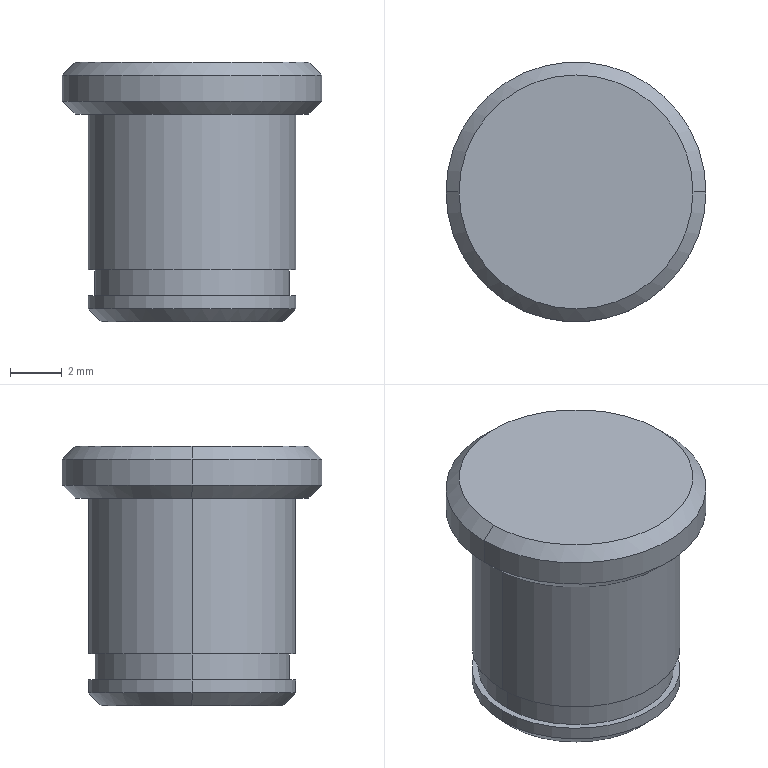Part | SolidWorks | features ICE 3, Chamfer 1, Extrusion 1 | 1 solid | 19 faces | box 10 x 10 x 10 mm | volume 542.514 mm3 | cylinder 8 | cone 6 | plane 5 | commonest cylinder face diameters 8 x4 7.5 x2 10 x2
STEP:
#1=CARTESIAN_POINT('',(4.5,0.,10.));
#2=VERTEX_POINT('',#1);
#3=CARTESIAN_POINT('',(-4.5,0.,10.));
#4=VERTEX_POINT('',#3);
#5=CARTESIAN_POINT('',(0.,0.,10.));
#6=DIRECTION('',(0.,0.,1.));
#7=DIRECTION('',(1.,0.,0.));
#8=AXIS2_PLACEMENT_3D('',#5,#6,#7);
#9=CIRCLE('',#8,4.5);
#10=EDGE_CURVE('',#2,#4,#9,.T.);
#11=ORIENTED_EDGE('',*,*,#10,.F.);
#12=CARTESIAN_POINT('',(5.,0.,9.5));
#13=VERTEX_POINT('',#12);
#14=CARTESIAN_POINT('',(4.5,0.,10.));
#15=DIRECTION('',(0.7071,0.,-0.7071));
#16=VECTOR('',#15,1000.);
#17=LINE('',#14,#16);
#18=EDGE_CURVE('',#2,#13,#17,.T.);
#19=ORIENTED_EDGE('',*,*,#18,.T.);
#20=CARTESIAN_POINT('',(-5.,0.,9.5));
#21=VERTEX_POINT('',#20);
#22=CARTESIAN_POINT('',(0.,0.,9.5));
#23=DIRECTION('',(0.,0.,-1.));
#24=DIRECTION('',(1.,0.,0.));
#25=AXIS2_PLACEMENT_3D('',#22,#23,#24);
#26=CIRCLE('',#25,5.);
#27=EDGE_CURVE('',#21,#13,#26,.T.);
#28=ORIENTED_EDGE('',*,*,#27,.F.);
#29=CARTESIAN_POINT('',(-4.5,0.,10.));
#30=DIRECTION('',(-0.7071,0.,-0.7071));
#31=VECTOR('',#30,1000.);
#32=LINE('',#29,#31);
#33=EDGE_CURVE('',#4,#21,#32,.T.);
#34=ORIENTED_EDGE('',*,*,#33,.F.);
#35=EDGE_LOOP('',(#11,#19,#28,#34));
#36=FACE_OUTER_BOUND('',#35,.T.);
#37=CARTESIAN_POINT('',(0.,0.,10.));
#38=DIRECTION('',(0.,0.,-1.));
#39=DIRECTION('',(-1.,0.,0.));
#40=AXIS2_PLACEMENT_3D('',#37,#38,#39);
#41=CONICAL_SURFACE('',#40,4.5,0.7854);
#42=ADVANCED_FACE('',(#36),#41,.T.);
#43=CARTESIAN_POINT('',(-4.5,0.,8.));
#44=VERTEX_POINT('',#43);
#45=CARTESIAN_POINT('',(4.5,0.,8.));
#46=VERTEX_POINT('',#45);
#47=CARTESIAN_POINT('',(0.,0.,8.));
#48=DIRECTION('',(0.,0.,-1.));
#49=DIRECTION('',(1.,0.,0.));
#50=AXIS2_PLACEMENT_3D('',#47,#48,#49);
#51=CIRCLE('',#50,4.5);
#52=EDGE_CURVE('',#44,#46,#51,.T.);
#53=ORIENTED_EDGE('',*,*,#52,.F.);
#54=CARTESIAN_POINT('',(-5.,0.,8.5));
#55=VERTEX_POINT('',#54);
#56=CARTESIAN_POINT('',(-5.,0.,8.5));
#57=DIRECTION('',(-0.7071,0.,0.7071));
#58=VECTOR('',#57,1000.);
#59=LINE('',#56,#58);
#60=EDGE_CURVE('',#44,#55,#59,.T.);
#61=ORIENTED_EDGE('',*,*,#60,.T.);
#62=CARTESIAN_POINT('',(5.,0.,8.5));
#63=VERTEX_POINT('',#62);
#64=CARTESIAN_POINT('',(0.,0.,8.5));
#65=DIRECTION('',(0.,0.,1.));
#66=DIRECTION('',(1.,0.,0.));
#67=AXIS2_PLACEMENT_3D('',#64,#65,#66);
#68=CIRCLE('',#67,5.);
#69=EDGE_CURVE('',#63,#55,#68,.T.);
#70=ORIENTED_EDGE('',*,*,#69,.F.);
#71=CARTESIAN_POINT('',(5.,0.,8.5));
#72=DIRECTION('',(0.7071,0.,0.7071));
#73=VECTOR('',#72,1000.);
#74=LINE('',#71,#73);
#75=EDGE_CURVE('',#46,#63,#74,.T.);
#76=ORIENTED_EDGE('',*,*,#75,.F.);
#77=EDGE_LOOP('',(#53,#61,#70,#76));
#78=FACE_OUTER_BOUND('',#77,.T.);
#79=CARTESIAN_POINT('',(0.,0.,8.5));
#80=DIRECTION('',(0.,0.,1.));
#81=DIRECTION('',(1.,0.,0.));
#82=AXIS2_PLACEMENT_3D('',#79,#80,#81);
#83=CONICAL_SURFACE('',#82,5.,0.7854);
#84=ADVANCED_FACE('',(#78),#83,.T.);
#85=CARTESIAN_POINT('',(-3.5,0.,0.));
#86=VERTEX_POINT('',#85);
#87=CARTESIAN_POINT('',(3.5,0.,0.));
#88=VERTEX_POINT('',#87);
#89=CARTESIAN_POINT('',(0.,0.,0.));
#90=DIRECTION('',(0.,0.,-1.));
#91=DIRECTION('',(1.,0.,0.));
#92=AXIS2_PLACEMENT_3D('',#89,#90,#91);
#93=CIRCLE('',#92,3.5);
#94=EDGE_CURVE('',#86,#88,#93,.T.);
#95=ORIENTED_EDGE('',*,*,#94,.F.);
#96=CARTESIAN_POINT('',(-4.,0.,0.5));
#97=VERTEX_POINT('',#96);
#98=CARTESIAN_POINT('',(-4.,0.,0.5));
#99=DIRECTION('',(-0.7071,0.,0.7071));
#100=VECTOR('',#99,1000.);
#101=LINE('',#98,#100);
#102=EDGE_CURVE('',#86,#97,#101,.T.);
#103=ORIENTED_EDGE('',*,*,#102,.T.);
#104=CARTESIAN_POINT('',(4.,0.,0.5));
#105=VERTEX_POINT('',#104);
#106=CARTESIAN_POINT('',(0.,0.,0.5));
#107=DIRECTION('',(0.,0.,1.));
#108=DIRECTION('',(1.,0.,0.));
#109=AXIS2_PLACEMENT_3D('',#106,#107,#108);
#110=CIRCLE('',#109,4.);
#111=EDGE_CURVE('',#105,#97,#110,.T.);
#112=ORIENTED_EDGE('',*,*,#111,.F.);
#113=CARTESIAN_POINT('',(4.,0.,0.5));
#114=DIRECTION('',(0.7071,0.,0.7071));
#115=VECTOR('',#114,1000.);
#116=LINE('',#113,#115);
#117=EDGE_CURVE('',#88,#105,#116,.T.);
#118=ORIENTED_EDGE('',*,*,#117,.F.);
#119=EDGE_LOOP('',(#95,#103,#112,#118));
#120=FACE_OUTER_BOUND('',#119,.T.);
#121=CARTESIAN_POINT('',(0.,0.,0.5));
#122=DIRECTION('',(0.,0.,1.));
#123=DIRECTION('',(1.,0.,0.));
#124=AXIS2_PLACEMENT_3D('',#121,#122,#123);
#125=CONICAL_SURFACE('',#124,4.,0.7854);
#126=ADVANCED_FACE('',(#120),#125,.T.);
#127=ORIENTED_EDGE('',*,*,#27,.T.);
#128=CARTESIAN_POINT('',(5.,0.,10.));
#129=DIRECTION('',(0.,0.,-1.));
#130=VECTOR('',#129,1000.);
#131=LINE('',#128,#130);
#132=EDGE_CURVE('',#13,#63,#131,.T.);
#133=ORIENTED_EDGE('',*,*,#132,.T.);
#134=ORIENTED_EDGE('',*,*,#69,.T.);
#135=CARTESIAN_POINT('',(-5.,0.,10.));
#136=DIRECTION('',(0.,0.,-1.));
#137=VECTOR('',#136,1000.);
#138=LINE('',#135,#137);
#139=EDGE_CURVE('',#21,#55,#138,.T.);
#140=ORIENTED_EDGE('',*,*,#139,.F.);
#141=EDGE_LOOP('',(#127,#133,#134,#140));
#142=FACE_OUTER_BOUND('',#141,.T.);
#143=CARTESIAN_POINT('',(0.,0.,10.));
#144=DIRECTION('',(0.,0.,-1.));
#145=DIRECTION('',(-1.,0.,0.));
#146=AXIS2_PLACEMENT_3D('',#143,#144,#145);
#147=CYLINDRICAL_SURFACE('',#146,5.);
#148=ADVANCED_FACE('',(#142),#147,.T.);
#149=CARTESIAN_POINT('',(4.,0.,8.));
#150=VERTEX_POINT('',#149);
#151=CARTESIAN_POINT('',(-4.,0.,8.));
#152=VERTEX_POINT('',#151);
#153=CARTESIAN_POINT('',(0.,0.,8.));
#154=DIRECTION('',(0.,0.,1.));
#155=DIRECTION('',(1.,0.,0.));
#156=AXIS2_PLACEMENT_3D('',#153,#154,#155);
#157=CIRCLE('',#156,4.);
#158=EDGE_CURVE('',#150,#152,#157,.T.);
#159=ORIENTED_EDGE('',*,*,#158,.F.);
#160=CARTESIAN_POINT('',(4.,0.,2.));
#161=VERTEX_POINT('',#160);
#162=CARTESIAN_POINT('',(4.,0.,8.));
#163=DIRECTION('',(0.,0.,-1.));
#164=VECTOR('',#163,1000.);
#165=LINE('',#162,#164);
#166=EDGE_CURVE('',#150,#161,#165,.T.);
#167=ORIENTED_EDGE('',*,*,#166,.T.);
#168=CARTESIAN_POINT('',(-4.,0.,2.));
#169=VERTEX_POINT('',#168);
#170=CARTESIAN_POINT('',(0.,0.,2.));
#171=DIRECTION('',(0.,0.,1.));
#172=DIRECTION('',(1.,0.,0.));
#173=AXIS2_PLACEMENT_3D('',#170,#171,#172);
#174=CIRCLE('',#173,4.);
#175=EDGE_CURVE('',#161,#169,#174,.T.);
#176=ORIENTED_EDGE('',*,*,#175,.T.);
#177=CARTESIAN_POINT('',(-4.,0.,8.));
#178=DIRECTION('',(0.,0.,-1.));
#179=VECTOR('',#178,1000.);
#180=LINE('',#177,#179);
#181=EDGE_CURVE('',#152,#169,#180,.T.);
#182=ORIENTED_EDGE('',*,*,#181,.F.);
#183=EDGE_LOOP('',(#159,#167,#176,#182));
#184=FACE_OUTER_BOUND('',#183,.T.);
#185=CARTESIAN_POINT('',(0.,0.,8.));
#186=DIRECTION('',(0.,0.,-1.));
#187=DIRECTION('',(-1.,0.,0.));
#188=AXIS2_PLACEMENT_3D('',#185,#186,#187);
#189=CYLINDRICAL_SURFACE('',#188,4.);
#190=ADVANCED_FACE('',(#184),#189,.T.);
#191=CARTESIAN_POINT('',(3.75,0.,2.));
#192=VERTEX_POINT('',#191);
#193=CARTESIAN_POINT('',(-3.75,0.,2.));
#194=VERTEX_POINT('',#193);
#195=CARTESIAN_POINT('',(0.,0.,2.));
#196=DIRECTION('',(0.,0.,1.));
#197=DIRECTION('',(1.,0.,0.));
#198=AXIS2_PLACEMENT_3D('',#195,#196,#197);
#199=CIRCLE('',#198,3.75);
#200=EDGE_CURVE('',#192,#194,#199,.T.);
#201=ORIENTED_EDGE('',*,*,#200,.F.);
#202=CARTESIAN_POINT('',(3.75,0.,1.));
#203=VERTEX_POINT('',#202);
#204=CARTESIAN_POINT('',(3.75,0.,2.));
#205=DIRECTION('',(0.,0.,-1.));
#206=VECTOR('',#205,1000.);
#207=LINE('',#204,#206);
#208=EDGE_CURVE('',#192,#203,#207,.T.);
#209=ORIENTED_EDGE('',*,*,#208,.T.);
#210=CARTESIAN_POINT('',(-3.75,0.,1.));
#211=VERTEX_POINT('',#210);
#212=CARTESIAN_POINT('',(0.,0.,1.));
#213=DIRECTION('',(0.,0.,1.));
#214=DIRECTION('',(1.,0.,0.));
#215=AXIS2_PLACEMENT_3D('',#212,#213,#214);
#216=CIRCLE('',#215,3.75);
#217=EDGE_CURVE('',#203,#211,#216,.T.);
#218=ORIENTED_EDGE('',*,*,#217,.T.);
#219=CARTESIAN_POINT('',(-3.75,0.,2.));
#220=DIRECTION('',(0.,0.,-1.));
#221=VECTOR('',#220,1000.);
#222=LINE('',#219,#221);
#223=EDGE_CURVE('',#194,#211,#222,.T.);
#224=ORIENTED_EDGE('',*,*,#223,.F.);
#225=EDGE_LOOP('',(#201,#209,#218,#224));
#226=FACE_OUTER_BOUND('',#225,.T.);
#227=CARTESIAN_POINT('',(0.,0.,2.));
#228=DIRECTION('',(0.,0.,-1.));
#229=DIRECTION('',(-1.,0.,0.));
#230=AXIS2_PLACEMENT_3D('',#227,#228,#229);
#231=CYLINDRICAL_SURFACE('',#230,3.75);
#232=ADVANCED_FACE('',(#226),#231,.T.);
#233=CARTESIAN_POINT('',(4.,0.,1.));
#234=VERTEX_POINT('',#233);
#235=CARTESIAN_POINT('',(-4.,0.,1.));
#236=VERTEX_POINT('',#235);
#237=CARTESIAN_POINT('',(0.,0.,1.));
#238=DIRECTION('',(0.,0.,1.));
#239=DIRECTION('',(1.,0.,0.));
#240=AXIS2_PLACEMENT_3D('',#237,#238,#239);
#241=CIRCLE('',#240,4.);
#242=EDGE_CURVE('',#234,#236,#241,.T.);
#243=ORIENTED_EDGE('',*,*,#242,.F.);
#244=CARTESIAN_POINT('',(4.,0.,1.));
#245=DIRECTION('',(0.,0.,-1.));
#246=VECTOR('',#245,1000.);
#247=LINE('',#244,#246);
#248=EDGE_CURVE('',#234,#105,#247,.T.);
#249=ORIENTED_EDGE('',*,*,#248,.T.);
#250=ORIENTED_EDGE('',*,*,#111,.T.);
#251=CARTESIAN_POINT('',(-4.,0.,1.));
#252=DIRECTION('',(0.,0.,-1.));
#253=VECTOR('',#252,1000.);
#254=LINE('',#251,#253);
#255=EDGE_CURVE('',#236,#97,#254,.T.);
#256=ORIENTED_EDGE('',*,*,#255,.F.);
#257=EDGE_LOOP('',(#243,#249,#250,#256));
#258=FACE_OUTER_BOUND('',#257,.T.);
#259=CARTESIAN_POINT('',(0.,0.,1.));
#260=DIRECTION('',(0.,0.,-1.));
#261=DIRECTION('',(-1.,0.,0.));
#262=AXIS2_PLACEMENT_3D('',#259,#260,#261);
#263=CYLINDRICAL_SURFACE('',#262,4.);
#264=ADVANCED_FACE('',(#258),#263,.T.);
#265=ORIENTED_EDGE('',*,*,#248,.F.);
#266=CARTESIAN_POINT('',(0.,0.,1.));
#267=DIRECTION('',(0.,0.,1.));
#268=DIRECTION('',(1.,0.,0.));
#269=AXIS2_PLACEMENT_3D('',#266,#267,#268);
#270=CIRCLE('',#269,4.);
#271=EDGE_CURVE('',#236,#234,#270,.T.);
#272=ORIENTED_EDGE('',*,*,#271,.F.);
#273=ORIENTED_EDGE('',*,*,#255,.T.);
#274=CARTESIAN_POINT('',(0.,0.,0.5));
#275=DIRECTION('',(0.,0.,1.));
#276=DIRECTION('',(1.,0.,0.));
#277=AXIS2_PLACEMENT_3D('',#274,#275,#276);
#278=CIRCLE('',#277,4.);
#279=EDGE_CURVE('',#97,#105,#278,.T.);
#280=ORIENTED_EDGE('',*,*,#279,.T.);
#281=EDGE_LOOP('',(#265,#272,#273,#280));
#282=FACE_OUTER_BOUND('',#281,.T.);
#283=CARTESIAN_POINT('',(0.,0.,1.));
#284=DIRECTION('',(0.,0.,-1.));
#285=DIRECTION('',(-1.,0.,0.));
#286=AXIS2_PLACEMENT_3D('',#283,#284,#285);
#287=CYLINDRICAL_SURFACE('',#286,4.);
#288=ADVANCED_FACE('',(#282),#287,.T.);
#289=CARTESIAN_POINT('',(0.,0.,1.));
#290=DIRECTION('',(0.,0.,1.));
#291=DIRECTION('',(1.,0.,0.));
#292=AXIS2_PLACEMENT_3D('',#289,#290,#291);
#293=CIRCLE('',#292,3.75);
#294=EDGE_CURVE('',#211,#203,#293,.T.);
#295=ORIENTED_EDGE('',*,*,#294,.F.);
#296=ORIENTED_EDGE('',*,*,#217,.F.);
#297=EDGE_LOOP('',(#295,#296));
#298=FACE_BOUND('',#297,.T.);
#299=ORIENTED_EDGE('',*,*,#271,.T.);
#300=ORIENTED_EDGE('',*,*,#242,.T.);
#301=EDGE_LOOP('',(#299,#300));
#302=FACE_OUTER_BOUND('',#301,.T.);
#303=CARTESIAN_POINT('',(0.,0.,1.));
#304=DIRECTION('',(0.,0.,1.));
#305=DIRECTION('',(1.,0.,0.));
#306=AXIS2_PLACEMENT_3D('',#303,#304,#305);
#307=PLANE('',#306);
#308=ADVANCED_FACE('',(#298,#302),#307,.T.);
#309=CARTESIAN_POINT('',(0.,0.,0.));
#310=DIRECTION('',(0.,0.,-1.));
#311=DIRECTION('',(1.,0.,0.));
#312=AXIS2_PLACEMENT_3D('',#309,#310,#311);
#313=CIRCLE('',#312,3.5);
#314=EDGE_CURVE('',#88,#86,#313,.T.);
#315=ORIENTED_EDGE('',*,*,#314,.T.);
#316=ORIENTED_EDGE('',*,*,#94,.T.);
#317=EDGE_LOOP('',(#315,#316));
#318=FACE_OUTER_BOUND('',#317,.T.);
#319=CARTESIAN_POINT('',(0.,0.,0.));
#320=DIRECTION('',(0.,0.,1.));
#321=DIRECTION('',(1.,0.,0.));
#322=AXIS2_PLACEMENT_3D('',#319,#320,#321);
#323=PLANE('',#322);
#324=ADVANCED_FACE('',(#318),#323,.F.);
#325=ORIENTED_EDGE('',*,*,#208,.F.);
#326=CARTESIAN_POINT('',(0.,0.,2.));
#327=DIRECTION('',(0.,0.,1.));
#328=DIRECTION('',(1.,0.,0.));
#329=AXIS2_PLACEMENT_3D('',#326,#327,#328);
#330=CIRCLE('',#329,3.75);
#331=EDGE_CURVE('',#194,#192,#330,.T.);
#332=ORIENTED_EDGE('',*,*,#331,.F.);
#333=ORIENTED_EDGE('',*,*,#223,.T.);
#334=ORIENTED_EDGE('',*,*,#294,.T.);
#335=EDGE_LOOP('',(#325,#332,#333,#334));
#336=FACE_OUTER_BOUND('',#335,.T.);
#337=CARTESIAN_POINT('',(0.,0.,2.));
#338=DIRECTION('',(0.,0.,-1.));
#339=DIRECTION('',(-1.,0.,0.));
#340=AXIS2_PLACEMENT_3D('',#337,#338,#339);
#341=CYLINDRICAL_SURFACE('',#340,3.75);
#342=ADVANCED_FACE('',(#336),#341,.T.);
#343=ORIENTED_EDGE('',*,*,#166,.F.);
#344=CARTESIAN_POINT('',(0.,0.,8.));
#345=DIRECTION('',(0.,0.,1.));
#346=DIRECTION('',(1.,0.,0.));
#347=AXIS2_PLACEMENT_3D('',#344,#345,#346);
#348=CIRCLE('',#347,4.);
#349=EDGE_CURVE('',#152,#150,#348,.T.);
#350=ORIENTED_EDGE('',*,*,#349,.F.);
#351=ORIENTED_EDGE('',*,*,#181,.T.);
#352=CARTESIAN_POINT('',(0.,0.,2.));
#353=DIRECTION('',(0.,0.,1.));
#354=DIRECTION('',(1.,0.,0.));
#355=AXIS2_PLACEMENT_3D('',#352,#353,#354);
#356=CIRCLE('',#355,4.);
#357=EDGE_CURVE('',#169,#161,#356,.T.);
#358=ORIENTED_EDGE('',*,*,#357,.T.);
#359=EDGE_LOOP('',(#343,#350,#351,#358));
#360=FACE_OUTER_BOUND('',#359,.T.);
#361=CARTESIAN_POINT('',(0.,0.,8.));
#362=DIRECTION('',(0.,0.,-1.));
#363=DIRECTION('',(-1.,0.,0.));
#364=AXIS2_PLACEMENT_3D('',#361,#362,#363);
#365=CYLINDRICAL_SURFACE('',#364,4.);
#366=ADVANCED_FACE('',(#360),#365,.T.);
#367=ORIENTED_EDGE('',*,*,#331,.T.);
#368=ORIENTED_EDGE('',*,*,#200,.T.);
#369=EDGE_LOOP('',(#367,#368));
#370=FACE_BOUND('',#369,.T.);
#371=ORIENTED_EDGE('',*,*,#357,.F.);
#372=ORIENTED_EDGE('',*,*,#175,.F.);
#373=EDGE_LOOP('',(#371,#372));
#374=FACE_OUTER_BOUND('',#373,.T.);
#375=CARTESIAN_POINT('',(0.,0.,2.));
#376=DIRECTION('',(0.,0.,1.));
#377=DIRECTION('',(1.,0.,0.));
#378=AXIS2_PLACEMENT_3D('',#375,#376,#377);
#379=PLANE('',#378);
#380=ADVANCED_FACE('',(#370,#374),#379,.F.);
#381=ORIENTED_EDGE('',*,*,#132,.F.);
#382=CARTESIAN_POINT('',(0.,0.,9.5));
#383=DIRECTION('',(0.,0.,-1.));
#384=DIRECTION('',(1.,0.,0.));
#385=AXIS2_PLACEMENT_3D('',#382,#383,#384);
#386=CIRCLE('',#385,5.);
#387=EDGE_CURVE('',#13,#21,#386,.T.);
#388=ORIENTED_EDGE('',*,*,#387,.T.);
#389=ORIENTED_EDGE('',*,*,#139,.T.);
#390=CARTESIAN_POINT('',(0.,0.,8.5));
#391=DIRECTION('',(0.,0.,1.));
#392=DIRECTION('',(1.,0.,0.));
#393=AXIS2_PLACEMENT_3D('',#390,#391,#392);
#394=CIRCLE('',#393,5.);
#395=EDGE_CURVE('',#55,#63,#394,.T.);
#396=ORIENTED_EDGE('',*,*,#395,.T.);
#397=EDGE_LOOP('',(#381,#388,#389,#396));
#398=FACE_OUTER_BOUND('',#397,.T.);
#399=CARTESIAN_POINT('',(0.,0.,10.));
#400=DIRECTION('',(0.,0.,-1.));
#401=DIRECTION('',(-1.,0.,0.));
#402=AXIS2_PLACEMENT_3D('',#399,#400,#401);
#403=CYLINDRICAL_SURFACE('',#402,5.);
#404=ADVANCED_FACE('',(#398),#403,.T.);
#405=CARTESIAN_POINT('',(0.,0.,10.));
#406=DIRECTION('',(0.,0.,1.));
#407=DIRECTION('',(1.,0.,0.));
#408=AXIS2_PLACEMENT_3D('',#405,#406,#407);
#409=CIRCLE('',#408,4.5);
#410=EDGE_CURVE('',#4,#2,#409,.T.);
#411=ORIENTED_EDGE('',*,*,#410,.T.);
#412=ORIENTED_EDGE('',*,*,#10,.T.);
#413=EDGE_LOOP('',(#411,#412));
#414=FACE_OUTER_BOUND('',#413,.T.);
#415=CARTESIAN_POINT('',(0.,0.,10.));
#416=DIRECTION('',(0.,0.,1.));
#417=DIRECTION('',(1.,0.,0.));
#418=AXIS2_PLACEMENT_3D('',#415,#416,#417);
#419=PLANE('',#418);
#420=ADVANCED_FACE('',(#414),#419,.T.);
#421=CARTESIAN_POINT('',(0.,0.,8.));
#422=DIRECTION('',(0.,0.,-1.));
#423=DIRECTION('',(1.,0.,0.));
#424=AXIS2_PLACEMENT_3D('',#421,#422,#423);
#425=CIRCLE('',#424,4.5);
#426=EDGE_CURVE('',#46,#44,#425,.T.);
#427=ORIENTED_EDGE('',*,*,#426,.T.);
#428=ORIENTED_EDGE('',*,*,#52,.T.);
#429=EDGE_LOOP('',(#427,#428));
#430=FACE_OUTER_BOUND('',#429,.T.);
#431=ORIENTED_EDGE('',*,*,#349,.T.);
#432=ORIENTED_EDGE('',*,*,#158,.T.);
#433=EDGE_LOOP('',(#431,#432));
#434=FACE_BOUND('',#433,.T.);
#435=CARTESIAN_POINT('',(0.,0.,8.));
#436=DIRECTION('',(0.,0.,1.));
#437=DIRECTION('',(1.,0.,0.));
#438=AXIS2_PLACEMENT_3D('',#435,#436,#437);
#439=PLANE('',#438);
#440=ADVANCED_FACE('',(#430,#434),#439,.F.);
#441=ORIENTED_EDGE('',*,*,#102,.F.);
#442=ORIENTED_EDGE('',*,*,#314,.F.);
#443=ORIENTED_EDGE('',*,*,#117,.T.);
#444=ORIENTED_EDGE('',*,*,#279,.F.);
#445=EDGE_LOOP('',(#441,#442,#443,#444));
#446=FACE_OUTER_BOUND('',#445,.T.);
#447=CARTESIAN_POINT('',(0.,0.,0.5));
#448=DIRECTION('',(0.,0.,1.));
#449=DIRECTION('',(1.,0.,0.));
#450=AXIS2_PLACEMENT_3D('',#447,#448,#449);
#451=CONICAL_SURFACE('',#450,4.,0.7854);
#452=ADVANCED_FACE('',(#446),#451,.T.);
#453=ORIENTED_EDGE('',*,*,#60,.F.);
#454=ORIENTED_EDGE('',*,*,#426,.F.);
#455=ORIENTED_EDGE('',*,*,#75,.T.);
#456=ORIENTED_EDGE('',*,*,#395,.F.);
#457=EDGE_LOOP('',(#453,#454,#455,#456));
#458=FACE_OUTER_BOUND('',#457,.T.);
#459=CARTESIAN_POINT('',(0.,0.,8.5));
#460=DIRECTION('',(0.,0.,1.));
#461=DIRECTION('',(1.,0.,0.));
#462=AXIS2_PLACEMENT_3D('',#459,#460,#461);
#463=CONICAL_SURFACE('',#462,5.,0.7854);
#464=ADVANCED_FACE('',(#458),#463,.T.);
#465=ORIENTED_EDGE('',*,*,#18,.F.);
#466=ORIENTED_EDGE('',*,*,#410,.F.);
#467=ORIENTED_EDGE('',*,*,#33,.T.);
#468=ORIENTED_EDGE('',*,*,#387,.F.);
#469=EDGE_LOOP('',(#465,#466,#467,#468));
#470=FACE_OUTER_BOUND('',#469,.T.);
#471=CARTESIAN_POINT('',(0.,0.,10.));
#472=DIRECTION('',(0.,0.,-1.));
#473=DIRECTION('',(-1.,0.,0.));
#474=AXIS2_PLACEMENT_3D('',#471,#472,#473);
#475=CONICAL_SURFACE('',#474,4.5,0.7854);
#476=ADVANCED_FACE('',(#470),#475,.T.);
#477=CLOSED_SHELL('',(#42,#84,#126,#148,#190,#232,#264,#288,#308,#324,#342,#366,#380,#404,#420,#440,#452,#464,#476));
#478=MANIFOLD_SOLID_BREP('',#477);
#479=CARTESIAN_POINT('',(0.,0.,0.));
#480=DIRECTION('',(0.,0.,1.));
#481=DIRECTION('',(1.,0.,0.));
#482=AXIS2_PLACEMENT_3D('',#479,#480,#481);
#483=(LENGTH_UNIT()NAMED_UNIT(*)SI_UNIT(.MILLI.,.METRE.));
#484=UNCERTAINTY_MEASURE_WITH_UNIT(LENGTH_MEASURE(0.00001),#483,'','');
#485=(NAMED_UNIT(*)PLANE_ANGLE_UNIT()SI_UNIT($,.RADIAN.));
#486=(NAMED_UNIT(*)SI_UNIT($,.STERADIAN.)SOLID_ANGLE_UNIT());
#487=(GEOMETRIC_REPRESENTATION_CONTEXT(3)GLOBAL_UNCERTAINTY_ASSIGNED_CONTEXT((#484))GLOBAL_UNIT_ASSIGNED_CONTEXT((#483,#485,#486))REPRESENTATION_CONTEXT('',''));
#488=ADVANCED_BREP_SHAPE_REPRESENTATION('',(#478,#482),#487);